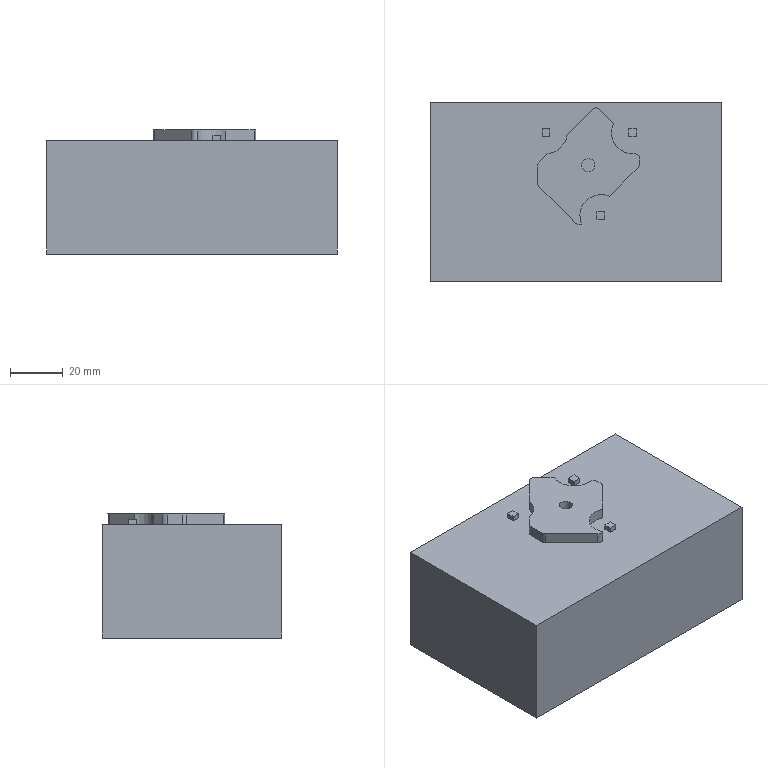NC program | NX | posted with a generic post | part box 110.151 x 68.163 x 47.1 mm
Lines 1 to 1466 of 32691:
N10 G17 G21 G94 G90
(FACE_MILLING , TOOL : E63)
N12 T01 M6
N14 G54
N16 G17 G0 G90 X93.875 Y-25.527 S3000 M3
N18 G43 Z83. H1
N20 G94 G1 Z0. F5000.
N22 X87.575 F1500.
N24 X-87.575
N26 Y25.527
N28 X87.575
N30 X93.875
N32 G0 Z83.
(PLANAR_PROFILE_2 , TOOL : E63)
N34 X-94.025 Y-25.581 S5000
N36 Z80.
N38 G1 Z-2. F5000.
N40 X-53.075 F1800.
N42 X53.075
N44 X94.025
N46 G0 Z-4.
N48 G1 X53.075
N50 X-53.075
N52 X-94.025
N54 G0 Z-6.
N56 G1 X-53.075
N58 X53.075
N60 X94.025
N62 G0 Z-8.
N64 G1 X53.075
N66 X-53.075
N68 X-94.025
N70 G0 Z-10.
N72 G1 X-53.075
N74 X53.075
N76 X94.025
N78 G0 Z-12.
N80 G1 X53.075
N82 X-53.075
N84 X-94.025
N86 G0 Z-14.
N88 G1 X-53.075
N90 X53.075
N92 X94.025
N94 G0 Z-16.
N96 G1 X53.075
N98 X-53.075
N100 X-94.025
N102 G0 Z-18.
N104 G1 X-53.075
N106 X53.075
N108 X94.025
N110 G0 Z-20.
N112 G1 X53.075
N114 X-53.075
N116 X-94.025
N118 G0 Z-22.
N120 G1 X-53.075
N122 X53.075
N124 X94.025
N126 G0 Z-24.
N128 G1 X53.075
N130 X-53.075
N132 X-94.025
N134 G0 Z-26.
N136 G1 X-53.075
N138 X53.075
N140 X94.025
N142 G0 Z-28.
N144 G1 X53.075
N146 X-53.075
N148 X-94.025
N150 G0 Z-30.
N152 G1 X-53.075
N154 X53.075
N156 X94.025
N158 G0 Z-32.
N160 G1 X53.075
N162 X-53.075
N164 X-94.025
N166 G0 Z-34.
N168 G1 X-53.075
N170 X53.075
N172 X94.025
N174 G0 Z80.
(ZLEVEL_PROFILE_STEEP , TOOL : E63)
N176 Z81.
N178 X48.517 Y75.021
N180 G1 Z-0.997 F5000.
N182 X48.524 Y43.521 F3000.
N184 X48.528 Y28.713
N186 G2 X16.009 Y-3.814 R32.519
N188 G1 X-25.958
N190 G2 X-58.478 Y28.713 R32.519
N192 G1 X-58.474 Y43.521
N194 X-58.466 Y75.021
N196 G0 Z81.
N198 X48.516
N200 G1 Z-1.994 F5000.
N202 X48.524 Y43.521 F3000.
N204 X48.528 Y28.638
N206 G2 X15.998 Y-3.901 R32.53
N208 G1 X-25.948
N210 G2 X-58.478 Y28.638 R32.53
N212 G1 X-58.474 Y43.521
N214 X-58.466 Y75.021
N216 G0 Z81.
N218 X48.516
N220 G1 Z-2.991 F5000.
N222 X48.524 Y43.521 F3000.
N224 X48.528 Y28.557
N226 G2 X15.992 Y-3.987 R32.536
N228 G1 X-25.941
N230 G2 X-58.478 Y28.558 R32.537
N232 G1 X-58.474 Y43.521
N234 X-58.466 Y75.021
N236 G0 Z81.
N238 X48.516
N240 G1 Z-3.988 F5000.
N242 X48.524 Y43.521 F3000.
N244 X48.528 Y28.47
N246 G2 X15.932 Y-4.075 R32.537
N248 G3 X-25.882 Y-4.075 R11354.304
N250 G2 X-58.478 Y28.47 R32.536
N252 G1 X-58.474 Y43.521
N254 X-58.466 Y75.021
N256 G0 Z81.
N258 X48.517
N260 G1 Z-4.985 F5000.
N262 X48.524 Y43.521 F3000.
N264 X48.528 Y28.384
N266 G2 X15.924 Y-4.162 R32.537
N268 G3 X-25.874 Y-4.161 R10089.369
N270 G2 X-58.478 Y28.384 R32.537
N272 G1 X-58.474 Y43.521
N274 X-58.466 Y75.021
N276 G0 Z81.
N278 X48.517
N280 G1 Z-5.982 F5000.
N282 X48.524 Y43.521 F3000.
N284 X48.528 Y28.727
N286 G2 X15.48 Y-4.247 R32.54
N288 G3 X-25.429 Y-4.247 R8682.147
N290 G2 X-58.478 Y28.727 R32.542
N292 G1 X-58.474 Y43.521
N294 X-58.466 Y75.021
N296 G0 Z81.
N298 X48.517
N300 G1 Z-6.979 F5000.
N302 X48.524 Y43.521 F3000.
N304 X48.528 Y28.212
N306 G2 X15.9 Y-4.335 R32.539
N308 G3 X-25.862 Y-4.335 R7619.424
N310 G2 X-58.478 Y28.2 R32.527
N312 G1 X-58.474 Y43.521
N314 X-58.466 Y75.021
N316 G0 Z81.
N318 X48.517
N320 G1 Z-7.976 F5000.
N322 X48.524 Y43.521 F3000.
N324 X48.528 Y28.127
N326 G2 X15.887 Y-4.422 R32.541
N328 G3 X-25.861 Y-4.422 R6788.492
N330 G2 X-58.339 Y25.213 R32.505
N332 X-58.478 Y28.727 R36.005
N334 G1 X-58.474 Y43.521
N336 X-58.467 Y75.021
N338 G0 Z81.
N340 X48.517
N342 G1 Z-8.974 F5000.
N344 X48.525 Y43.521 F3000.
N346 X48.528 Y28.04
N348 G2 X15.876 Y-4.509 R32.541
N350 G3 X-25.851 Y-4.509 R6120.973
N352 G2 X-58.337 Y25.114 R32.504
N354 X-58.478 Y28.727 R36.269
N356 G1 X-58.474 Y43.521
N358 X-58.467 Y75.021
N360 G0 Z81.
N362 X48.517
N364 G1 Z-9.971 F5000.
N366 X48.525 Y43.521 F3000.
N368 X48.528 Y27.928
N370 G2 X15.89 Y-4.596 R32.516
N372 G3 X-25.843 Y-4.596 R5572.978
N374 G2 X-58.423 Y26.319 R32.496
N376 X-58.478 Y28.727 R46.78
N378 G1 X-58.474 Y43.521
N380 X-58.467 Y75.021
N382 G0 Z81.
N384 X48.517
N386 G1 Z-10.968 F5000.
N388 X48.525 Y43.521 F3000.
N390 X48.528 Y27.85
N392 G2 X15.881 Y-4.682 R32.525
N394 G3 X-25.842 Y-4.682 R5540.967
N396 G2 X-58.427 Y26.327 R32.496
N398 X-58.478 Y28.727 R49.042
N400 G1 X-58.474 Y43.521
N402 X-58.467 Y75.021
N404 G0 Z81.
N406 X48.517
N408 G1 Z-11.965 F5000.
N410 X48.525 Y43.521 F3000.
N412 X48.528 Y28.727
N414 X48.515 Y27.41
N416 G2 X15.998 Y-4.768 R32.497
N418 G1 X11.584 Y-4.765
N420 X-4.001 Y-4.71
N422 X-5.949
N424 X-21.533 Y-4.765
N426 X-25.429 Y-4.767
N428 X-26.523 Y-4.75
N430 G2 X-58.454 Y27.201 R32.459
N432 G1 X-58.478 Y28.727
N434 X-58.474 Y43.521
N436 X-58.467 Y75.021
N438 G0 Z81.
N440 X48.517
N442 G1 Z-12.962 F5000.
N444 X48.525 Y43.521 F3000.
N446 X48.528 Y28.727
N448 X48.516 Y27.355
N450 G2 X15.998 Y-4.855 R32.496
N452 G1 X11.584 Y-4.851
N454 X-4.001 Y-4.792
N456 X-5.949
N458 X-21.533 Y-4.851
N460 X-25.429 Y-4.854
N462 X-26.522 Y-4.837
N464 G2 X-58.456 Y27.16 R32.46
N466 G1 X-58.478 Y28.727
N468 X-58.474 Y43.521
N470 X-58.467 Y75.021
N472 G0 Z81.
N474 X48.517
N476 G1 Z-13.959 F5000.
N478 X48.525 Y43.521 F3000.
N480 X48.528 Y28.727
N482 X48.517 Y27.299
N484 G2 X16. Y-4.941 R32.494
N486 G1 X11.584 Y-4.938
N488 X-4.001 Y-4.874
N490 X-5.949
N492 X-21.533 Y-4.938
N494 X-25.961 Y-4.941
N496 G2 X-58.457 Y27.119 R32.476
N498 G1 X-58.478 Y28.727
N500 X-58.474 Y43.521
N502 X-58.467 Y75.021
N504 G0 Z81.
N506 X48.517
N508 G1 Z-14.956 F5000.
N510 X48.525 Y43.521 F3000.
N512 X48.528 Y28.727
N514 X48.518 Y27.245
N516 G2 X16. Y-5.028 R32.493
N518 G1 X11.584 Y-5.024
N520 X-4.001 Y-4.955
N522 X-5.949
N524 X-21.533 Y-5.024
N526 X-25.929 Y-5.028
N528 G2 X-58.459 Y27.108 R32.507
N530 G1 X-58.478 Y28.727
N532 X-58.474 Y43.521
N534 X-58.467 Y75.021
N536 G0 Z81.
N538 X48.517
N540 G1 Z-15.953 F5000.
N542 X48.525 Y43.521 F3000.
N544 X48.528 Y28.727
N546 X48.519 Y27.218
N548 G2 X15.973 Y-5.115 R32.52
N550 G1 X11.584 Y-5.111
N552 X-4.001 Y-5.037
N554 X-5.949
N556 X-21.533 Y-5.111
N558 X-25.93 Y-5.115
N560 G2 X-58.461 Y27.065 R32.507
N562 G1 X-58.478 Y28.727
N564 X-58.474 Y43.521
N566 X-58.467 Y75.021
N568 G0 Z81.
N570 X48.517
N572 G1 Z-16.95 F5000.
N574 X48.525 Y43.521 F3000.
N576 X48.528 Y28.727
N578 X48.521 Y27.166
N580 G2 X15.97 Y-5.201 R32.523
N582 G1 X11.584 Y-5.198
N584 X-4.001 Y-5.119
N586 X-25.429 Y-5.201
N588 G2 X-58.461 Y26.756 R32.511
N590 G1 X-58.478 Y28.727
N592 X-58.474 Y43.521
N594 X-58.467 Y75.021
N596 G0 Z81.
N598 X48.517
N600 G1 Z-17.947 F5000.
N602 X48.525 Y43.521 F3000.
N604 X48.528 Y28.727
N606 X48.522 Y27.118
N608 G2 X15.965 Y-5.288 R32.528
N610 G1 X11.584 Y-5.284
N612 X-4.001 Y-5.201
N614 X-25.429 Y-5.288
N616 G2 X-58.463 Y26.756 R32.517
N618 G1 X-58.478 Y28.727
N620 X-58.474 Y43.521
N622 X-58.467 Y75.021
N624 G0 Z81.
N626 X48.517
N628 G1 Z-18.944 F5000.
N630 X48.525 Y43.521 F3000.
N632 X48.528 Y28.727
N634 X48.524 Y27.067
N636 G2 X15.963 Y-5.375 R32.531
N638 G1 X11.584 Y-5.371
N640 X-4.001 Y-5.282
N642 X-25.429 Y-5.374
N644 G2 X-58.466 Y26.756 R32.521
N646 G1 X-58.478 Y28.727
N648 X-58.475 Y43.521
N650 X-58.467 Y75.021
N652 G0 Z81.
N654 X48.517
N656 G1 Z-19.941 F5000.
N658 X48.525 Y43.521 F3000.
N660 X48.528 Y28.727
N662 X48.525 Y27.014
N664 G2 X15.976 Y-5.461 R32.532
N666 G1 X13.532 Y-5.46
N668 X-4.001 Y-5.364
N670 X-5.949
N672 X-23.481 Y-5.46
N674 X-25.929 Y-5.461
N676 G2 X-58.469 Y26.912 R32.523
N678 G1 X-58.478 Y28.727
N680 X-58.475 Y43.521
N682 X-58.467 Y75.021
N684 G0 Z81.
N686 X48.518
N688 G1 Z-20.938 F5000.
N690 X48.525 Y43.521 F3000.
N692 X48.528 Y28.727
N694 X48.526 Y26.949
N696 G2 X15.978 Y-5.548 R32.53
N698 G1 X13.532 Y-5.547
N700 X-4.001 Y-5.446
N702 X-5.949
N704 X-23.481 Y-5.546
N706 X-25.931 Y-5.548
N708 G2 X-58.472 Y26.869 R32.522
N710 G1 X-58.478 Y28.727
N712 X-58.475 Y43.521
N714 X-58.468 Y75.021
N716 G0 Z81.
N718 X48.518
N720 G1 Z-21.935 F5000.
N722 X48.525 Y43.521 F3000.
N724 X48.528 Y28.727
N726 X48.526 Y26.866
N728 G2 X15.975 Y-5.635 R32.532
N730 G1 X13.532 Y-5.633
N732 X-4.001 Y-5.528
N734 X-5.949
N736 X-23.481 Y-5.633
N738 X-25.926 Y-5.635
N740 G2 X-58.474 Y26.834 R32.529
N742 G1 X-58.478 Y28.727
N744 X-58.475 Y43.521
N746 X-58.468 Y75.021
N748 G0 Z81.
N750 X48.518
N752 G1 Z-22.932 F5000.
N754 X48.525 Y43.521 F3000.
N756 X48.528 Y28.727
N758 X48.526 Y26.783
N760 G2 X15.972 Y-5.721 R32.534
N762 G1 X13.532 Y-5.72
N764 X-4.001 Y-5.609
N766 X-5.949
N768 X-23.481 Y-5.72
N770 X-25.922 Y-5.721
N772 G2 X-58.477 Y26.819 R32.536
N774 G1 X-58.475 Y43.521
N776 X-58.47 Y75.021
N778 G0 Z81.
N780 X48.518
N782 G1 Z-23.929 F5000.
N784 X48.525 Y43.521 F3000.
N786 X48.528 Y28.727
N788 X48.526 Y26.698
N790 G2 X15.971 Y-5.808 R32.535
N792 G1 X13.532 Y-5.806
N794 X-0.105 Y-5.71
N796 G3 X-11.793 Y-5.731 R586.138
N798 G1 X-15.689 Y-5.765
N800 X-17.637 Y-5.775
N802 X-25.429 Y-5.808
N804 G2 X-58.478 Y26.756 R32.538
N806 G1 X-58.475 Y43.521
N808 X-58.469 Y75.021
N810 G0 Z81.
N812 X48.522
N814 G1 Z-24.926 F5000.
N816 X48.525 Y43.521 F3000.
N818 X48.527 Y26.643
N820 G2 X15.98 Y-5.895 R32.534
N822 X-0.105 Y-5.793 R1356.4
N824 G3 X-11.793 Y-5.814 R568.568
N826 G1 X-15.689 Y-5.85
N828 X-17.637 Y-5.861
N830 X-25.429 Y-5.894
N832 G2 X-58.478 Y26.756 R32.537
N834 G1 X-58.475 Y43.521
N836 X-58.469 Y75.021
N838 G0 Z81.
N840 X48.522
N842 G1 Z-25.924 F5000.
N844 X48.525 Y43.521 F3000.
N846 X48.527 Y26.553
N848 G2 X15.961 Y-5.982 R32.531
N850 X-0.105 Y-5.876 R1445.596
N852 G3 X-11.793 Y-5.897 R546.516
N854 G1 X-15.689 Y-5.935
N856 X-17.637 Y-5.946
N858 X-25.429 Y-5.981
N860 G2 X-58.478 Y26.756 R32.534
N862 G1 X-58.475 Y43.521
N864 X-58.469 Y75.021
N866 G0 Z81.
N868 X48.521
N870 G1 Z-26.921 F5000.
N872 X48.525 Y43.521 F3000.
N874 X48.527 Y26.467
N876 G2 X15.961 Y-6.068 R32.531
N878 X-0.105 Y-5.958 R1382.623
N880 G3 X-11.793 Y-5.98 R526.111
N882 G1 X-15.689 Y-6.02
N884 X-17.637 Y-6.032
N886 X-25.429 Y-6.068
N888 G2 X-58.478 Y26.756 R32.535
N890 G1 X-58.475 Y43.521
N892 X-58.469 Y75.021
N894 G0 Z81.
N896 X48.521
N898 G1 Z-27.918 F5000.
N900 X48.525 Y43.521 F3000.
N902 X48.527 Y26.381
N904 G2 X15.96 Y-6.155 R32.533
N906 X-0.105 Y-6.041 R1324.909
N908 G3 X-11.793 Y-6.064 R507.174
N910 G1 X-15.689 Y-6.105
N912 X-17.637 Y-6.117
N914 X-25.429 Y-6.154
N916 G2 X-58.478 Y26.756 R32.536
N918 G1 X-58.475 Y43.521
N920 X-58.469 Y75.021
N922 G0 Z81.
N924 X48.521
N926 G1 Z-28.915 F5000.
N928 X48.525 Y43.521 F3000.
N930 X48.527 Y26.294
N932 G2 X15.961 Y-6.242 R32.532
N934 X0.889 Y-6.137 R1271.755
N936 G3 X-9.661 Y-6.125 R447.39
N938 G1 X-15.689 Y-6.19
N940 X-17.637 Y-6.203
N942 X-25.782 Y-6.243
N944 G2 X-58.478 Y26.298 R32.535
N946 G1 X-58.475 Y43.521
N948 X-58.469 Y75.021
N950 G0 Z81.
N952 X48.521
N954 G1 Z-29.912 F5000.
N956 X48.525 Y43.521 F3000.
N958 X48.527 Y26.208
N960 G2 X15.962 Y-6.329 R32.532
N962 X0.86 Y-6.22 R1221.66
N964 G3 X-9.548 Y-6.207 R426.995
N966 G1 X-15.689 Y-6.275
N968 X-23.481 Y-6.326
N970 X-25.918 Y-6.328
N972 G2 X-58.478 Y26.211 R32.533
N974 G1 X-58.475 Y43.521
N976 X-58.469 Y75.021
N978 G0 Z81.
N980 X48.521
N982 G1 Z-30.909 F5000.
N984 X48.525 Y43.521 F3000.
N986 X48.527 Y26.118
N988 G2 X15.971 Y-6.415 R32.529
N990 G1 X13.532 Y-6.413
N992 X3.791 Y-6.338
N994 X0.393 Y-6.295
N996 G3 X-9.463 Y-6.289 R414.767
N998 G1 X-15.689 Y-6.36
N1000 X-23.481 Y-6.413
N1002 X-25.921 Y-6.415
N1004 G2 X-58.478 Y26.121 R32.53
N1006 G1 X-58.475 Y43.521
N1008 X-58.469 Y75.021
N1010 G0 Z81.
N1012 X48.521
N1014 G1 Z-31.906 F5000.
N1016 X48.525 Y43.521 F3000.
N1018 X48.527 Y26.001
N1020 G2 X16.001 Y-6.502 R32.499
N1022 G1 X13.532 Y-6.5
N1024 X3.791 Y-6.422
N1026 X-0.105 Y-6.372
N1028 G3 X-9.845 Y-6.372 R452.112
N1030 G1 X-13.741 Y-6.422
N1032 X-23.481 Y-6.5
N1034 X-25.951 Y-6.502
N1036 G2 X-58.478 Y26.004 R32.499
N1038 G1 X-58.475 Y43.521
N1040 X-58.469 Y75.021
N1042 G0 Z81.
N1044 X48.521 Y75.005
N1046 G1 Z-32.903 F5000.
N1048 X48.525 Y43.505 F3000.
N1050 X48.527 Y26.756
N1052 X48.506 Y24.786
N1054 G2 X17.428 Y-6.575 R32.535
N1056 X3.791 Y-6.507 R660.092
N1058 G3 X-13.741 Y-6.506 R502.73
N1060 G2 X-25.429 Y-6.588 R842.455
N1062 G1 X-27.377 Y-6.557
N1064 G2 X-58.457 Y24.786 R32.484
N1066 G1 X-58.478 Y26.756
N1068 X-58.475 Y43.521
N1070 X-58.469 Y75.021
N1072 G0 Z81.
N1074 X48.521 Y75.005
N1076 G1 Z-33.9 F5000.
N1078 X48.525 Y43.505 F3000.
N1080 X48.527 Y26.756
N1082 X48.517 Y25.524
N1084 G2 X16.08 Y-6.704 R32.5
N1086 X3.791 Y-6.63 R778.625
N1088 G3 X-13.741 Y-6.63 R491.142
N1090 G2 X-26.028 Y-6.704 R780.361
N1092 X-58.469 Y25.537 R32.502
N1094 G1 X-58.478 Y26.756
N1096 X-58.475 Y43.505
N1098 X-58.468 Y75.005
N1100 G0 Z81.
N1102 M5
(FACE_MILLING_1_COPY_1 , TOOL : D25R0)
N1104 T02 M6
N1106 G54
N1108 G17 G0 G90 X-17.475 Y59.9 S6000 M3
N1110 G43 Z10. H2
N1112 G94 G1 Z-0.4 F5000.
N1114 G3 X-4.975 Y47.4 R12.5 F2500.
N1116 G1 X15.025
N1118 G2 X24.147 Y43.622 R12.9
N1120 G1 X25.147 Y42.622
N1122 G2 X28.925 Y33.5 R12.9
N1124 G1 Y28.74
N1126 G2 X16.025 Y15.84 R12.9
N1128 G1 X-25.975
N1130 G2 X-38.875 Y28.74 R12.9
N1132 G1 Y33.5
N1134 G2 X-35.097 Y42.622 R12.9
N1136 G1 X-34.097 Y43.622
N1138 G2 X-24.975 Y47.4 R12.9
N1140 G1 X-4.975
N1142 G3 X7.525 Y59.9 R12.5
N1144 G0 X-17.475 Z-2.8
N1146 G3 X-4.975 Y47.4 R12.5
N1148 G1 X15.025
N1150 G2 X24.147 Y43.622 R12.9
N1152 G1 X25.147 Y42.622
N1154 G2 X28.925 Y33.5 R12.9
N1156 G1 Y28.531
N1158 G2 X16.025 Y15.631 R12.9
N1160 G1 X-25.975
N1162 G2 X-38.875 Y28.531 R12.9
N1164 G1 Y33.5
N1166 G2 X-35.097 Y42.622 R12.9
N1168 G1 X-34.097 Y43.622
N1170 G2 X-24.975 Y47.4 R12.9
N1172 G1 X-4.975
N1174 G3 X7.525 Y59.9 R12.5
N1176 G0 X-17.475 Z-5.2
N1178 G3 X-4.975 Y47.4 R12.5
N1180 G1 X15.025
N1182 G2 X24.147 Y43.622 R12.9
N1184 G1 X25.147 Y42.622
N1186 G2 X28.925 Y33.5 R12.9
N1188 G1 Y28.322
N1190 G2 X16.025 Y15.422 R12.9
N1192 G1 X2.357
N1194 X-3.422 Y15.565
N1196 X-8.769 Y15.532
N1198 X-10.594 Y15.485
N1200 X-12.299 Y15.422
N1202 X-25.975
N1204 G2 X-38.875 Y28.322 R12.9
N1206 G1 Y33.5
N1208 G2 X-35.097 Y42.622 R12.9
N1210 G1 X-34.097 Y43.622
N1212 G2 X-24.975 Y47.4 R12.9
N1214 G1 X-4.975
N1216 G3 X7.525 Y59.9 R12.5
N1218 G0 X-17.475 Z-7.6
N1220 G3 X-4.975 Y47.4 R12.5
N1222 G1 X15.025
N1224 G2 X24.147 Y43.622 R12.9
N1226 G1 X25.147 Y42.622
N1228 G2 X28.925 Y33.5 R12.9
N1230 G1 Y28.114
N1232 G2 X16.025 Y15.214 R12.9
N1234 G1 X5.894
N1236 G3 X-4.974 Y15.571 R161.394
N1238 X-15.843 Y15.214 R161.304
N1240 G1 X-25.975
N1242 G2 X-38.875 Y28.114 R12.9
N1244 G1 Y33.5
N1246 G2 X-35.097 Y42.622 R12.9
N1248 G1 X-34.097 Y43.622
N1250 G2 X-24.975 Y47.4 R12.9
N1252 G1 X-4.975
N1254 G3 X7.525 Y59.9 R12.5
N1256 G0 X-17.475 Z-10.
N1258 G3 X-4.975 Y47.4 R12.5
N1260 G1 X15.025
N1262 G2 X24.147 Y43.622 R12.9
N1264 G1 X25.147 Y42.622
N1266 G2 X28.925 Y33.5 R12.9
N1268 G1 Y27.905
N1270 G2 X16.025 Y15.005 R12.9
N1272 G1 X8.048
N1274 X6.188 Y15.183
N1276 G3 X-4.963 Y15.571 R157.925
N1278 G1 X-6.888 Y15.561
N1280 G3 X-17.971 Y15.005 R132.546
N1282 G1 X-25.975
N1284 G2 X-38.875 Y27.905 R12.9
N1286 G1 Y33.5
N1288 G2 X-35.097 Y42.622 R12.9
N1290 G1 X-34.097 Y43.622
N1292 G2 X-24.975 Y47.4 R12.9
N1294 G1 X-4.975
N1296 G3 X7.525 Y59.9 R12.5
N1298 G0 X-17.475 Z-12.4
N1300 G3 X-4.975 Y47.4 R12.5
N1302 G1 X15.025
N1304 G2 X24.147 Y43.622 R12.9
N1306 G1 X25.147 Y42.622
N1308 G2 X28.925 Y33.5 R12.9
N1310 G1 Y27.696
N1312 G2 X16.025 Y14.796 R12.9
N1314 G1 X9.422
N1316 X7.643 Y15.037
N1318 X6.673 Y15.14
N1320 G3 X-4.944 Y15.571 R157.19
N1322 G1 X-10.587 Y15.485
N1324 X-12.309 Y15.42
N1326 G3 X-19.256 Y14.796 R68.691
N1328 G1 X-25.975
N1330 G2 X-38.875 Y27.696 R12.9
N1332 G1 Y33.5
N1334 G2 X-35.097 Y42.622 R12.9
N1336 G1 X-34.097 Y43.622
N1338 G2 X-24.975 Y47.4 R12.9
N1340 G1 X-4.975
N1342 G3 X7.525 Y59.9 R12.5
N1344 G0 X-17.475 Z-14.8
N1346 G3 X-4.975 Y47.4 R12.5
N1348 G1 X15.025
N1350 G2 X24.147 Y43.622 R12.9
N1352 G1 X25.147 Y42.622
N1354 G2 X28.925 Y33.5 R12.9
N1356 G1 Y27.488
N1358 G2 X16.025 Y14.588 R12.9
N1360 G1 X10.162
N1362 X8.408 Y14.93
N1364 X7.874 Y15.008
N1366 X6.99 Y15.109
N1368 G3 X-4.953 Y15.571 R153.415
N1370 X-15.336 Y15.246 R161.477
N1372 X-19.974 Y14.588 R29.395
N1374 G1 X-25.975
N1376 G2 X-38.875 Y27.488 R12.9
N1378 G1 Y33.5
N1380 G2 X-35.097 Y42.622 R12.9
N1382 G1 X-34.097 Y43.622
N1384 G2 X-24.975 Y47.4 R12.9
N1386 G1 X-4.975
N1388 G3 X7.525 Y59.9 R12.5
N1390 G0 X-17.475 Z-17.2
N1392 G3 X-4.975 Y47.4 R12.5
N1394 G1 X15.025
N1396 G2 X24.147 Y43.622 R12.9
N1398 G1 X25.147 Y42.622
N1400 G2 X28.925 Y33.5 R12.9
N1402 G1 Y27.279
N1404 G2 X16.025 Y14.379 R12.9
N1406 G1 X10.177
N1408 X8.38 Y14.933
N1410 X8.029 Y14.988
N1412 X7.216 Y15.085
N1414 G3 X-4.961 Y15.571 R150.401
N1416 G1 X-10.587 Y15.485
N1418 G3 X-18.33 Y14.933 R90.218
N1420 G2 X-22.071 Y14.379 R12.9
N1422 G1 X-25.975
N1424 G2 X-38.875 Y27.279 R12.9
N1426 G1 Y33.5
N1428 G2 X-35.097 Y42.622 R12.9
N1430 G1 X-34.097 Y43.622
N1432 G2 X-24.975 Y47.4 R12.9
N1434 G1 X-4.975
N1436 G3 X7.525 Y59.9 R12.5
N1438 G0 X-17.475 Z-19.6
N1440 G3 X-4.975 Y47.4 R12.5
N1442 G1 X15.025
N1444 G2 X24.147 Y43.622 R12.9
N1446 G1 X25.147 Y42.622
N1448 G2 X28.925 Y33.5 R12.9
N1450 G1 Y27.07
N1452 G2 X16.025 Y14.17 R12.9
N1454 G1 X12.475
N1456 G2 X7.925 Y14.999 R12.9
N1458 G1 X7.394 Y15.066
N1460 G3 X-4.967 Y15.571 R147.81
N1462 G1 X-6.888 Y15.561
N1464 X-8.769 Y15.532
N1466 G3 X-17.876 Y14.999 R112.655
N1468 G2 X-22.424 Y14.17 R12.9
N1470 G1 X-25.975
N1472 G2 X-38.875 Y27.07 R12.9
N1474 G1 Y33.5
N1476 G2 X-35.097 Y42.622 R12.9
N1478 G1 X-34.097 Y43.622
N1480 G2 X-24.975 Y47.4 R12.9
N1482 G1 X-4.975
N1484 G3 X7.525 Y59.9 R12.5
N1486 G0 X-17.475 Z-22.
N1488 G3 X-4.975 Y47.4 R12.5
N1490 G1 X15.025
N1492 G2 X24.147 Y43.622 R12.9
N1494 G1 X25.147 Y42.622
N1496 G2 X28.925 Y33.5 R12.9
N1498 G1 Y26.861
N1500 G2 X16.025 Y13.961 R12.9
N1502 G1 X12.492
N1504 G2 X7.237 Y15.08 R12.9
N1506 G3 X-4.973 Y15.571 R147.388
N1508 X-17.187 Y15.08 R146.928
N1510 G2 X-22.441 Y13.961 R12.9
N1512 G1 X-25.975
N1514 G2 X-38.875 Y26.861 R12.9
N1516 G1 Y33.5
N1518 G2 X-35.097 Y42.622 R12.9
N1520 G1 X-34.097 Y43.622
N1522 G2 X-24.975 Y47.4 R12.9
N1524 G1 X-4.975
N1526 G3 X7.525 Y59.9 R12.5
N1528 G0 X-17.475 Z-24.4
N1530 G3 X-4.975 Y47.4 R12.5
N1532 G1 X15.025
N1534 G2 X24.147 Y43.622 R12.9
N1536 G1 X25.147 Y42.622
N1538 G2 X28.925 Y33.5 R12.9
N1540 G1 Y26.653
N1542 G2 X16.025 Y13.753 R12.9
N1544 G1 X12.174
N1546 G2 X6.287 Y15.174 R12.9
N1548 G3 X-16.242 Y15.172 R159.595
N1550 G2 X-22.123 Y13.753 R12.9
N1552 G1 X-25.975
N1554 G2 X-38.875 Y26.653 R12.9
N1556 G1 Y33.5
N1558 G2 X-35.097 Y42.622 R12.9
N1560 G1 X-34.097 Y43.622
N1562 G2 X-24.975 Y47.4 R12.9
N1564 G1 X-4.975
N1566 G3 X7.525 Y59.9 R12.5
N1568 G0 X-17.475 Z-26.8
N1570 G3 X-4.975 Y47.4 R12.5
N1572 G1 X15.025
N1574 G2 X24.147 Y43.622 R12.9
N1576 G1 X25.147 Y42.622
N1578 G2 X28.925 Y33.5 R12.9
N1580 G1 Y26.444
N1582 G2 X16.025 Y13.544 R12.9
N1584 G1 X11.501
N1586 G2 X5.055 Y15.27 R12.9
N1588 G3 X-4.968 Y15.571 R163.936
N1590 X-15.009 Y15.268 R161.789
N1592 G2 X-21.451 Y13.544 R12.9
N1594 G1 X-25.975
N1596 G2 X-38.875 Y26.444 R12.9
N1598 G1 Y33.5
N1600 G2 X-35.097 Y42.622 R12.9
N1602 G1 X-34.097 Y43.622
N1604 G2 X-24.975 Y47.4 R12.9
N1606 G1 X-4.975
N1608 G3 X7.525 Y59.9 R12.5
N1610 G0 X-17.475 Z-29.2
N1612 G3 X-4.975 Y47.4 R12.5
N1614 G1 X15.025
N1616 G2 X24.147 Y43.622 R12.9
N1618 G1 X25.147 Y42.622
N1620 G2 X28.925 Y33.5 R12.9
N1622 G1 Y26.235
N1624 G2 X16.025 Y13.335 R12.9
N1626 G1 X10.427
N1628 G2 X3.481 Y15.365 R12.9
N1630 G3 X-13.434 Y15.363 R173.032
N1632 G2 X-20.377 Y13.335 R12.9
N1634 G1 X-25.975
N1636 G2 X-38.875 Y26.235 R12.9
N1638 G1 Y33.5
N1640 G2 X-35.097 Y42.622 R12.9
N1642 G1 X-34.097 Y43.622
N1644 G2 X-24.975 Y47.4 R12.9
N1646 G1 X-4.975
N1648 G3 X7.525 Y59.9 R12.5
N1650 G0 X-17.475 Z-31.6
N1652 G3 X-4.975 Y47.4 R12.5
N1654 G1 X15.025
N1656 G2 X24.147 Y43.622 R12.9
N1658 G1 X25.147 Y42.622
N1660 G2 X28.925 Y33.5 R12.9
N1662 G1 Y26.027
N1664 G2 X16.025 Y13.127 R12.9
N1666 G1 X8.86
N1668 G2 X1.469 Y15.454 R12.9
N1670 G1 X-3.126 Y15.562
N1672 X-8.769 Y15.532
N1674 X-10.587 Y15.485
N1676 X-11.419 Y15.454
N1678 G2 X-18.81 Y13.127 R12.9
N1680 G1 X-25.975
N1682 G2 X-38.875 Y26.027 R12.9
N1684 G1 Y33.5
N1686 G2 X-35.097 Y42.622 R12.9
N1688 G1 X-34.097 Y43.622
N1690 G2 X-24.975 Y47.4 R12.9
N1692 G1 X-4.975
N1694 G3 X7.525 Y59.9 R12.5
N1696 G0 X-17.475 Z-34.
N1698 G3 X-4.975 Y47.4 R12.5
N1700 G1 X15.025
N1702 G2 X24.147 Y43.622 R12.9
N1704 G1 X25.147 Y42.622
N1706 G2 X28.925 Y33.5 R12.9
N1708 G1 Y25.786
N1710 G2 X16.025 Y12.886 R12.9
N1712 G1 X10.406
N1714 G2 X8.697 Y13. R12.9
N1716 G1 X6.614
N1718 G2 X-1.056 Y15.528 R12.9
N1720 G1 X-6.888 Y15.561
N1722 X-8.769 Y15.532
N1724 X-8.892 Y15.529
N1726 G2 X-16.564 Y13. R12.9
N1728 G1 X-18.646
N1730 G2 X-20.356 Y12.886 R12.9
N1732 G1 X-25.975
N1734 G2 X-38.875 Y25.786 R12.9
N1736 G1 Y33.5
N1738 G2 X-35.097 Y42.622 R12.9
N1740 G1 X-34.097 Y43.622
N1742 G2 X-24.975 Y47.4 R12.9
N1744 G1 X-4.975
N1746 G3 X7.525 Y59.9 R12.5
N1748 G0 Z10.
(PLANAR_MILL , TOOL : D25R0)
N1750 Z46.
N1752 X-73.375 Y-2.121
N1754 G1 Z-35.5 F5000.
N1756 X-65.875 F2500.
N1758 Y24.042
N1760 G2 X-62.126 Y33.093 R12.8
N1762 G1 X-44.087 Y51.132
N1764 G2 X-35.036 Y54.881 R12.8
N1766 G1 X29.328
N1768 G2 X38.379 Y51.132 R12.8
N1770 G1 X62.126 Y27.385
N1772 G2 X65.875 Y18.335 R12.8
N1774 G1 Y-14.092
N1776 G2 X62.126 Y-23.143 R12.8
N1778 G1 X34.137 Y-51.132
N1780 G2 X25.086 Y-54.881 R12.8
N1782 G1 X-39.278
N1784 G2 X-48.329 Y-51.132 R12.8
N1786 G1 X-62.126 Y-37.335
N1788 G2 X-65.875 Y-28.284 R12.8
N1790 G1 Y-2.121
N1792 X-73.375
N1794 G0 Z-37.
N1796 G1 X-65.875
N1798 Y24.042
N1800 G2 X-62.126 Y33.093 R12.8
N1802 G1 X-44.087 Y51.132
N1804 G2 X-35.036 Y54.881 R12.8
N1806 G1 X29.328
N1808 G2 X38.379 Y51.132 R12.8
N1810 G1 X62.126 Y27.385
N1812 G2 X65.875 Y18.335 R12.8
N1814 G1 Y-14.092
N1816 G2 X62.126 Y-23.143 R12.8
N1818 G1 X34.137 Y-51.132
N1820 G2 X25.086 Y-54.881 R12.8
N1822 G1 X-39.278
N1824 G2 X-48.329 Y-51.132 R12.8
N1826 G1 X-62.126 Y-37.335
N1828 G2 X-65.875 Y-28.284 R12.8
N1830 G1 Y-2.121
N1832 X-73.375
N1834 G0 Z-38.5
N1836 G1 X-65.875
N1838 Y24.042
N1840 G2 X-62.126 Y33.093 R12.8
N1842 G1 X-44.087 Y51.132
N1844 G2 X-35.036 Y54.881 R12.8
N1846 G1 X29.328
N1848 G2 X38.379 Y51.132 R12.8
N1850 G1 X62.126 Y27.385
N1852 G2 X65.875 Y18.335 R12.8
N1854 G1 Y-14.092
N1856 G2 X62.126 Y-23.143 R12.8
N1858 G1 X34.137 Y-51.132
N1860 G2 X25.086 Y-54.881 R12.8
N1862 G1 X-39.278
N1864 G2 X-48.329 Y-51.132 R12.8
N1866 G1 X-62.126 Y-37.335
N1868 G2 X-65.875 Y-28.284 R12.8
N1870 G1 Y-2.121
N1872 X-73.375
N1874 G0 Z-40.
N1876 G1 X-65.875
N1878 Y24.042
N1880 G2 X-62.126 Y33.093 R12.8
N1882 G1 X-44.087 Y51.132
N1884 G2 X-35.036 Y54.881 R12.8
N1886 G1 X29.328
N1888 G2 X38.379 Y51.132 R12.8
N1890 G1 X62.126 Y27.385
N1892 G2 X65.875 Y18.335 R12.8
N1894 G1 Y-14.092
N1896 G2 X62.126 Y-23.143 R12.8
N1898 G1 X34.137 Y-51.132
N1900 G2 X25.086 Y-54.881 R12.8
N1902 G1 X-39.278
N1904 G2 X-48.329 Y-51.132 R12.8
N1906 G1 X-62.126 Y-37.335
N1908 G2 X-65.875 Y-28.284 R12.8
N1910 G1 Y-2.121
N1912 X-73.375
N1914 G0 Z-41.5
N1916 G1 X-65.875
N1918 Y24.042
N1920 G2 X-62.126 Y33.093 R12.8
N1922 G1 X-44.087 Y51.132
N1924 G2 X-35.036 Y54.881 R12.8
N1926 G1 X29.328
N1928 G2 X38.379 Y51.132 R12.8
N1930 G1 X62.126 Y27.385
N1932 G2 X65.875 Y18.335 R12.8
N1934 G1 Y-14.092
N1936 G2 X62.126 Y-23.143 R12.8
N1938 G1 X34.137 Y-51.132
N1940 G2 X25.086 Y-54.881 R12.8
N1942 G1 X-39.278
N1944 G2 X-48.329 Y-51.132 R12.8
N1946 G1 X-62.126 Y-37.335
N1948 G2 X-65.875 Y-28.284 R12.8
N1950 G1 Y-2.121
N1952 X-73.375
N1954 G0 Z-43.
N1956 G1 X-65.875
N1958 Y24.042
N1960 G2 X-62.126 Y33.093 R12.8
N1962 G1 X-44.087 Y51.132
N1964 G2 X-35.036 Y54.881 R12.8
N1966 G1 X29.328
N1968 G2 X38.379 Y51.132 R12.8
N1970 G1 X62.126 Y27.385
N1972 G2 X65.875 Y18.335 R12.8
N1974 G1 Y-14.092
N1976 G2 X62.126 Y-23.143 R12.8
N1978 G1 X34.137 Y-51.132
N1980 G2 X25.086 Y-54.881 R12.8
N1982 G1 X-39.278
N1984 G2 X-48.329 Y-51.132 R12.8
N1986 G1 X-62.126 Y-37.335
N1988 G2 X-65.875 Y-28.284 R12.8
N1990 G1 Y-2.121
N1992 X-73.375
N1994 G0 Z-44.5
N1996 G1 X-65.875
N1998 Y24.042
N2000 G2 X-62.126 Y33.093 R12.8
N2002 G1 X-44.087 Y51.132
N2004 G2 X-35.036 Y54.881 R12.8
N2006 G1 X29.328
N2008 G2 X38.379 Y51.132 R12.8
N2010 G1 X62.126 Y27.385
N2012 G2 X65.875 Y18.335 R12.8
N2014 G1 Y-14.092
N2016 G2 X62.126 Y-23.143 R12.8
N2018 G1 X34.137 Y-51.132
N2020 G2 X25.086 Y-54.881 R12.8
N2022 G1 X-39.278
N2024 G2 X-48.329 Y-51.132 R12.8
N2026 G1 X-62.126 Y-37.335
N2028 G2 X-65.875 Y-28.284 R12.8
N2030 G1 Y-2.121
N2032 X-73.375
N2034 G0 Z-46.
N2036 G1 X-65.875
N2038 Y24.042
N2040 G2 X-62.126 Y33.093 R12.8
N2042 G1 X-44.087 Y51.132
N2044 G2 X-35.036 Y54.881 R12.8
N2046 G1 X29.328
N2048 G2 X38.379 Y51.132 R12.8
N2050 G1 X62.126 Y27.385
N2052 G2 X65.875 Y18.335 R12.8
N2054 G1 Y-14.092
N2056 G2 X62.126 Y-23.143 R12.8
N2058 G1 X34.137 Y-51.132
N2060 G2 X25.086 Y-54.881 R12.8
N2062 G1 X-39.278
N2064 G2 X-48.329 Y-51.132 R12.8
N2066 G1 X-62.126 Y-37.335
N2068 G2 X-65.875 Y-28.284 R12.8
N2070 G1 Y-2.121
N2072 X-73.375
N2074 G0 Z-47.5
N2076 G1 X-65.875
N2078 Y24.042
N2080 G2 X-62.126 Y33.093 R12.8
N2082 G1 X-44.087 Y51.132
N2084 G2 X-35.036 Y54.881 R12.8
N2086 G1 X29.328
N2088 G2 X38.379 Y51.132 R12.8
N2090 G1 X62.126 Y27.385
N2092 G2 X65.875 Y18.335 R12.8
N2094 G1 Y-14.092
N2096 G2 X62.126 Y-23.143 R12.8
N2098 G1 X34.137 Y-51.132
N2100 G2 X25.086 Y-54.881 R12.8
N2102 G1 X-39.278
N2104 G2 X-48.329 Y-51.132 R12.8
N2106 G1 X-62.126 Y-37.335
N2108 G2 X-65.875 Y-28.284 R12.8
N2110 G1 Y-2.121
N2112 X-73.375
N2114 G0 Z-48.8
N2116 G1 X-65.875
N2118 Y24.042
N2120 G2 X-62.126 Y33.093 R12.8
N2122 G1 X-44.087 Y51.132
N2124 G2 X-35.036 Y54.881 R12.8
N2126 G1 X29.328
N2128 G2 X38.379 Y51.132 R12.8
N2130 G1 X62.126 Y27.385
N2132 G2 X65.875 Y18.335 R12.8
N2134 G1 Y-14.092
N2136 G2 X62.126 Y-23.143 R12.8
N2138 G1 X34.137 Y-51.132
N2140 G2 X25.086 Y-54.881 R12.8
N2142 G1 X-39.278
N2144 G2 X-48.329 Y-51.132 R12.8
N2146 G1 X-62.126 Y-37.335
N2148 G2 X-65.875 Y-28.284 R12.8
N2150 G1 Y-2.121
N2152 X-73.375
N2154 G0 Z46.
(CAVITY_MILL_4 , TOOL : D25R0)
N2156 Z80.5
N2158 X-18.406 Y-60.009
N2160 G1 Z-35.5 F5000.
N2162 Y-55.009 F2500.
N2164 X-38.16 Y-55.01
N2166 X-39.598 Y-55.008
N2168 X-40.317 Y-54.975
N2170 X-41.037 Y-54.902
N2172 X-41.756 Y-54.789
N2174 X-42.475 Y-54.634
N2176 G2 X-46.072 Y-53.152 R13.024
N2178 X-49.088 Y-50.685 R14.973
N2180 G1 X-62.048 Y-37.725
N2182 X-62.596 Y-37.171
N2184 G2 X-66.186 Y-28.35 R13.02
N2186 G1 X-66.187 Y7.922
N2188 Y21.761
N2190 Y24.214
N2192 X-66.163 Y24.935
N2194 X-66.098 Y25.656
N2196 X-65.992 Y26.378
N2198 X-65.845 Y27.098
N2200 G2 X-62.126 Y33.588 R13.331
N2202 G1 X-44.639 Y51.075
N2204 X-44.12 Y51.59
N2206 G2 X-35.287 Y55.192 R13.039
N2208 G1 X29.357 Y55.193
N2210 G2 X32.954 Y54.651 R13.02
N2212 X38.709 Y51.114 R13.424
N2214 G1 X61.995 Y27.828
N2216 G2 X66.004 Y18.453 R13.178
N2218 G1 Y-13.949
N2220 G2 X62.073 Y-23.324 R13.084
N2222 G1 X34.399 Y-50.997
N2224 X33.986 Y-51.406
N2226 G2 X25.048 Y-55.009 R13.02
N2228 G1 X-17.993
N2230 X-18.406
N2232 X-18.407 Y-36.259
N2234 X-36.997 Y-36.26
N2236 X-47.436 Y-25.82
N2238 X-47.437 Y7.923
N2240 Y21.76
N2242 X-42.817 Y26.381
N2244 Y25.492
N2246 G3 X-26.067 Y8.742 R16.75
N2248 G1 X-21.567
N2250 G3 X-17.505 Y9.242 R16.75
N2252 G1 X-14.643
N2254 G3 X-13.054 Y9.321 R15.928
N2256 X-5.77 Y11.81 R16.931
N2258 G2 X-4.355 Y11.811 R178.974
N2260 G3 X-3.725 Y11.433 R16.512
N2262 G1 Y11.
N2264 G3 X13.025 Y-5.75 R16.75
N2266 G1 X16.025
N2268 G3 X32.775 Y11. R16.75
N2270 G1 Y14.
N2272 G3 X31.712 Y19.872 R16.75
N2274 X32.683 Y25.492 R16.75
N2276 G1 Y30.623
N2278 X28.933
N2280 Y25.876
N2282 Y25.814
N2284 Y25.492
N2286 G2 X27.64 Y19.839 R13.
N2288 X29.025 Y14. R13.
N2290 G1 Y11.
N2292 G2 X16.025 Y-2. R13.
N2294 G1 X13.025
N2296 G2 X0.025 Y11. R13.
N2298 G1 Y13.81
N2300 G2 X-3.184 Y15.551 R12.762
N2302 G3 X-3.97 Y15.559 R155.623
N2304 X-6.337 Y15.557 R182.724
N2306 X-6.932 Y15.551 R155.623
N2308 G2 X-13.428 Y13.053 R13.181
N2310 X-14.643 Y12.992 R12.178
N2312 G1 X-17.996
N2314 G2 X-21.567 Y12.492 R13.
N2316 G1 X-26.067
N2318 G2 X-39.067 Y25.492 R13.
N2320 G1 Y33.592
N2322 G2 X-34.741 Y43.274 R13.
N2324 G1 X-34.605 Y43.438
N2326 X-34.259 Y43.784
N2328 G2 X-25.067 Y47.592 R13.
N2330 G1 X14.933
N2332 G2 X24.126 Y43.784 R13.
N2334 G1 X24.47 Y43.44
N2336 X24.612 Y43.298
N2338 X24.609 Y43.273
N2340 X24.784 Y43.126
N2342 X25.126 Y42.784
N2344 G2 X28.933 Y33.592 R13.
N2346 G1 Y30.623
N2348 X32.683
N2350 X47.254 Y16.053
N2352 Y-11.626
N2354 X22.621 Y-36.259
N2356 X-8.128 Y-36.26
N2358 X-17.493 Y-36.259
N2360 X-18.407
N2362 Y-17.509
N2364 X-28.687
N2366 Y-9.911
N2368 G3 X-26.067 Y-10.008 R35.5
N2370 G1 X-21.567
N2372 G3 X-15.918 Y-9.556 R35.5
N2374 X-8.128 Y-17.51 R35.5
N2376 G1 X2.697 Y-23.759
N2378 X17.443
N2380 X24.085 Y-17.118
N2382 G2 X16.025 Y-18.25 R29.25
N2384 G1 X13.025
N2386 G2 X4.359 Y-16.937 R29.25
N2388 X2.697 Y-23.759 R12.5
N2390 G1 X-8.128 Y-17.51
N2392 X-16.993 Y-17.509
N2394 X-18.407
N2396 Y-22.509
N2398 G0 Z-33.7
N2400 X-18.406 Y-60.009
N2402 G1 Z-37. F5000.
N2404 Y-55.009 F2500.
N2406 X-38.16 Y-55.01
N2408 X-39.598 Y-55.008
N2410 X-40.317 Y-54.975
N2412 X-41.037 Y-54.902
N2414 X-41.756 Y-54.789
N2416 X-42.475 Y-54.634
N2418 G2 X-46.072 Y-53.152 R13.024
N2420 X-49.088 Y-50.685 R14.973
N2422 G1 X-62.048 Y-37.725
N2424 X-62.596 Y-37.171
N2426 G2 X-66.186 Y-28.35 R13.02
N2428 G1 X-66.187 Y7.922
N2430 Y21.761
N2432 Y24.214
N2434 X-66.163 Y24.935
N2436 X-66.098 Y25.656
N2438 X-65.992 Y26.378
N2440 X-65.845 Y27.098
N2442 G2 X-62.126 Y33.588 R13.331
N2444 G1 X-44.639 Y51.075
N2446 X-44.12 Y51.59
N2448 G2 X-35.287 Y55.192 R13.039
N2450 G1 X29.357 Y55.193
N2452 G2 X32.954 Y54.651 R13.02
N2454 X38.709 Y51.114 R13.424
N2456 G1 X61.995 Y27.828
N2458 G2 X66.004 Y18.453 R13.178
N2460 G1 Y-13.949
N2462 G2 X62.073 Y-23.324 R13.084
N2464 G1 X34.399 Y-50.997
N2466 X33.986 Y-51.406
N2468 G2 X25.048 Y-55.009 R13.02
N2470 G1 X-17.993
N2472 X-18.406
N2474 X-18.407 Y-36.259
N2476 X-36.997 Y-36.26
N2478 X-47.436 Y-25.82
N2480 X-47.437 Y7.923
N2482 Y21.76
N2484 X-42.817 Y26.381
N2486 Y25.492
N2488 G3 X-26.067 Y8.742 R16.75
N2490 G1 X-21.567
N2492 G3 X-17.505 Y9.242 R16.75
N2494 G1 X-11.898
N2496 G3 X-5.066 Y10.701 R16.717
N2498 X-3.793 Y10.193 R16.666
N2500 X1.135 Y-0.798 R16.75
N2502 X13.025 Y-5.75 R16.75
N2504 G1 X16.025
N2506 G3 X32.775 Y11. R16.75
N2508 G1 Y14.
N2510 G3 X31.712 Y19.872 R16.75
N2512 X32.683 Y25.492 R16.75
N2514 G1 Y30.623
N2516 X28.933
N2518 Y25.492
N2520 G2 X27.64 Y19.839 R13.
N2522 X29.025 Y14. R13.
N2524 G1 Y11.
N2526 G2 X16.025 Y-2. R13.
N2528 G1 X13.025
N2530 G2 X6.343 Y-0.151 R13.
N2532 G1 X6.309 Y-0.131
N2534 G2 X3.787 Y1.854 R13.
N2536 X-0.067 Y11.092 R13.
N2538 G1 Y13.123
N2540 G2 X-5.066 Y14.938 R12.916
N2542 X-11.898 Y12.992 R12.967
N2544 G1 X-17.996
N2546 G2 X-21.567 Y12.492 R13.
N2548 G1 X-26.067
N2550 G2 X-39.067 Y25.492 R13.
N2552 G1 Y33.592
N2554 G2 X-34.75 Y43.266 R13.
N2556 G1 X-34.755 Y43.289
N2558 X-34.606 Y43.437
N2560 X-34.259 Y43.784
N2562 G2 X-25.067 Y47.592 R13.
N2564 G1 X14.933
N2566 G2 X24.126 Y43.784 R13.
N2568 G1 X24.482 Y43.428
N2570 X24.612 Y43.298
N2572 X24.609 Y43.273
N2574 X24.784 Y43.126
N2576 X25.039 Y42.871
N2578 X25.126 Y42.784
N2580 G2 X28.933 Y33.592 R13.
N2582 G1 Y30.623
N2584 X32.683
N2586 X47.254 Y16.053
N2588 Y-11.626
N2590 X22.621 Y-36.259
N2592 X-8.128 Y-36.26
N2594 X-17.493 Y-36.259
N2596 X-18.407
N2598 Y-17.509
N2600 X-28.687
N2602 Y-9.911
N2604 G3 X-26.067 Y-10.008 R35.5
N2606 G1 X-21.567
N2608 G3 X-15.942 Y-9.56 R35.5
N2610 X-12.123 Y-14.056 R35.5
N2612 X-8.128 Y-17.51 R35.5
N2614 G1 X2.697 Y-23.759
N2616 X17.443
N2618 X24.085 Y-17.118
N2620 G2 X16.025 Y-18.25 R29.25
N2622 G1 X13.025
N2624 G2 X4.359 Y-16.937 R29.25
N2626 X2.697 Y-23.759 R12.5
N2628 G1 X-8.128 Y-17.51
N2630 X-16.993 Y-17.509
N2632 X-18.407
N2634 Y-22.509
N2636 G0 Z-35.2
N2638 X-18.406 Y-60.009
N2640 G1 Z-38. F5000.
N2642 Y-55.009 F2500.
N2644 X-38.16 Y-55.01
N2646 X-39.598 Y-55.008
N2648 X-40.317 Y-54.975
N2650 X-41.037 Y-54.902
N2652 X-41.756 Y-54.789
N2654 X-42.475 Y-54.634
N2656 G2 X-46.072 Y-53.152 R13.024
N2658 X-49.088 Y-50.685 R14.973
N2660 G1 X-62.048 Y-37.725
N2662 X-62.596 Y-37.171
N2664 G2 X-66.186 Y-28.35 R13.02
N2666 G1 X-66.187 Y7.922
N2668 Y21.761
N2670 Y24.214
N2672 X-66.163 Y24.935
N2674 X-66.098 Y25.656
N2676 X-65.992 Y26.378
N2678 X-65.845 Y27.098
N2680 G2 X-62.126 Y33.588 R13.331
N2682 G1 X-44.639 Y51.075
N2684 X-44.12 Y51.59
N2686 G2 X-35.287 Y55.192 R13.039
N2688 G1 X29.357 Y55.193
N2690 G2 X32.954 Y54.651 R13.02
N2692 X38.709 Y51.114 R13.424
N2694 G1 X61.995 Y27.828
N2696 G2 X66.004 Y18.453 R13.178
N2698 G1 Y-13.949
N2700 G2 X62.073 Y-23.324 R13.084
N2702 G1 X34.399 Y-50.997
N2704 X33.986 Y-51.406
N2706 G2 X25.048 Y-55.009 R13.02
N2708 G1 X-2.654 Y-55.01
N2710 Y-36.26
N2712 G3 X8.683 Y-20.408 R16.75
N2714 G1 Y-17.408
N2716 G3 X-8.129 Y-0.658 R16.75
N2718 X-5.067 Y3.638 R16.75
N2720 X9.933 Y-5.658 R16.75
N2722 G1 X11.273
N2724 G3 X11.723 Y-5.699 R16.75
N2726 X13.033 Y-5.75 R15.329
N2728 G1 X16.025
N2730 G3 X32.775 Y11. R16.75
N2732 G1 Y14.
N2734 G3 X31.712 Y19.872 R16.75
N2736 X32.683 Y25.492 R16.75
N2738 G1 Y30.623
N2740 X47.254 Y16.053
N2742 Y-11.626
N2744 X22.621 Y-36.259
N2746 X-2.654 Y-36.26
N2748 X19.796 Y-23.174
N2750 G3 X19.933 Y-20.408 R28.
N2752 G1 Y-17.408
N2754 G3 X19.925 Y-16.727 R28.
N2756 X29.337 Y-13.633 R28.
N2758 G1 X19.796 Y-23.174
N2760 X-2.654 Y-36.26
N2762 Y-55.01
N2764 X-17.993 Y-55.009
N2766 X-18.406
N2768 X-18.407 Y-36.259
N2770 X-36.997 Y-36.26
N2772 X-47.436 Y-25.82
N2774 X-47.437 Y7.923
N2776 Y21.76
N2778 X-42.817 Y26.381
N2780 Y25.492
N2782 G3 X-39.729 Y15.802 R16.75
N2784 X-39.817 Y14.092 R16.75
N2786 G1 Y11.092
N2788 G3 X-23.004 Y-5.658 R16.75
N2790 G1 Y-1.908
N2792 X-23.067
N2794 G2 X-36.067 Y11.092 R13.
N2796 G1 Y14.092
N2798 G2 X-35.772 Y16.843 R13.
N2800 X-39.067 Y25.492 R13.
N2802 G1 Y33.592
N2804 G2 X-34.75 Y43.266 R13.
N2806 G1 X-34.755 Y43.289
N2808 X-34.606 Y43.437
N2810 X-34.259 Y43.784
N2812 G2 X-25.067 Y47.592 R13.
N2814 G1 X14.933
N2816 G2 X24.126 Y43.784 R13.
N2818 G1 X24.481 Y43.429
N2820 X24.612 Y43.298
N2822 X24.609 Y43.273
N2824 X24.784 Y43.126
N2826 X25.125 Y42.785
N2828 G2 X28.933 Y33.592 R13.
N2830 G1 Y25.492
N2832 G2 X27.64 Y19.839 R13.
N2834 X29.025 Y14. R13.
N2836 G1 Y11.
N2838 G2 X16.025 Y-2. R13.
N2840 G1 X13.025
N2842 G2 X12.022 Y-1.961 R11.579
N2844 X11.482 Y-1.908 R13.
N2846 G1 X9.933
N2848 G2 X-3.067 Y11.092 R13.
N2850 G1 Y13.106
N2852 G2 X-5.066 Y13.534 R12.849
N2854 X-7.067 Y13.106 R12.823
N2856 G1 Y11.092
N2858 G2 X-20.067 Y-1.908 R13.
N2860 G1 X-23.004
N2862 Y-5.658
N2864 G3 X-27.817 Y-17.408 R16.75
N2866 G1 Y-20.408
N2868 G3 X-16.479 Y-36.26 R16.75
N2870 G1 X-15.267 Y-32.711
N2872 G2 X-24.067 Y-20.408 R13.
N2874 G1 Y-17.408
N2876 G2 X-11.067 Y-4.408 R13.
N2878 G1 X-8.067
N2880 G2 X4.933 Y-17.408 R13.
N2882 G1 Y-20.408
N2884 G2 X-8.067 Y-33.408 R13.
N2886 G1 X-11.067
N2888 G2 X-15.267 Y-32.711 R13.
N2890 G1 X-16.479 Y-36.26
N2892 X-17.493 Y-36.259
N2894 X-18.407
N2896 Y-41.259
N2898 G0 Z80.5
N2900 M5